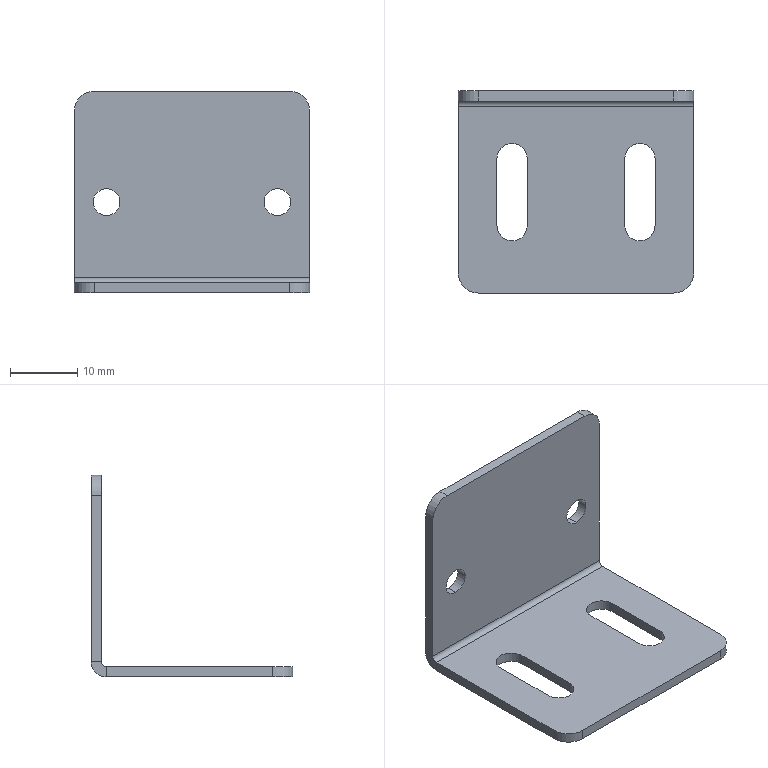Part | STEP file | PN_0038(Default) | 1 solid | 30 faces | box 35 x 30 x 30 mm | volume 2806 mm3 | plane 16 | cylinder 14 | commonest cylinder face diameters 4 x4 4.5 x4 6 x4 1.473 x1 4.473 x1